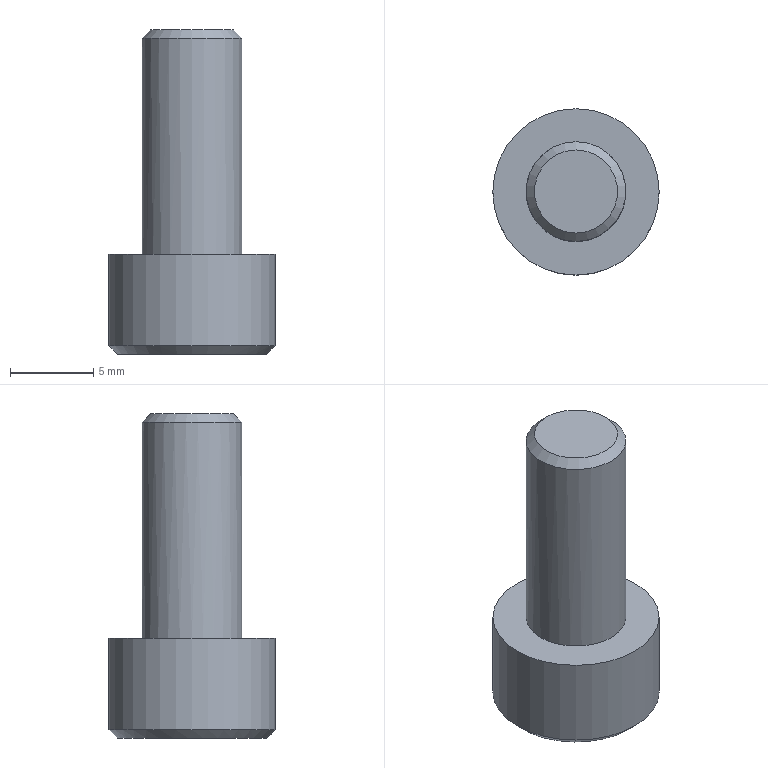Part | STEP file | solid 222 | 1 solid | 14 faces | box 10 x 10 x 19.5 mm | volume 781.969 mm3 | plane 10 | cone 2 | cylinder 2 | commonest cylinder face diameters 6 x1 10 x1